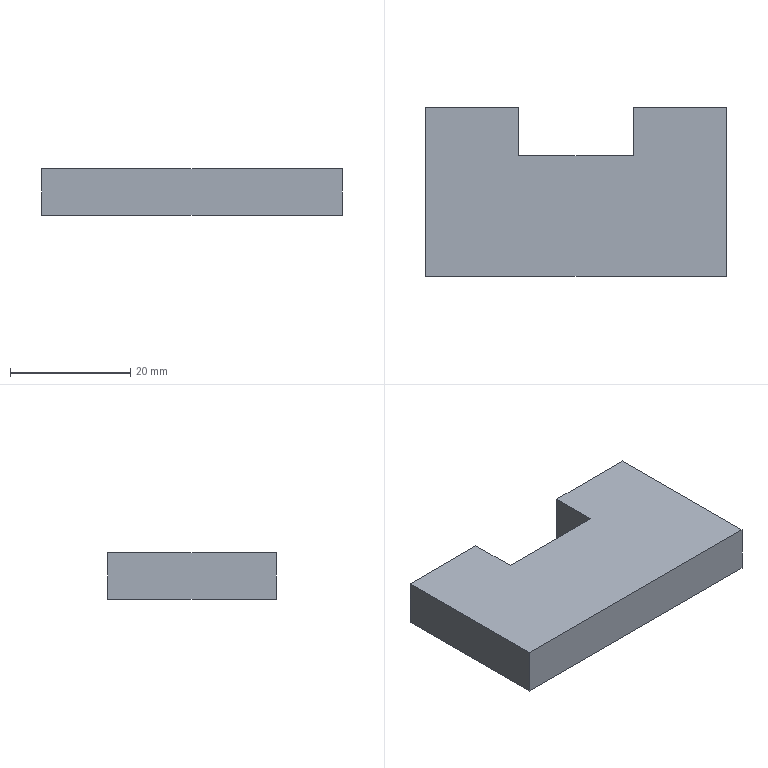Part | 1 solid | 10 faces | box 50 x 28 x 7.8 mm | volume 9734 mm3 | plane 10
STEP:
#1=CARTESIAN_POINT('',(25.,-14.,0.));
#2=VERTEX_POINT('',#1);
#3=CARTESIAN_POINT('',(25.,14.,0.));
#4=VERTEX_POINT('',#3);
#5=CARTESIAN_POINT('',(25.,14.,0.));
#6=DIRECTION('',(0.,1.,0.));
#7=VECTOR('',#6,1000.);
#8=LINE('',#5,#7);
#9=EDGE_CURVE('',#2,#4,#8,.T.);
#10=ORIENTED_EDGE('',*,*,#9,.F.);
#11=CARTESIAN_POINT('',(25.,-14.,-7.8));
#12=VERTEX_POINT('',#11);
#13=CARTESIAN_POINT('',(25.,-14.,-7.8));
#14=DIRECTION('',(0.,0.,1.));
#15=VECTOR('',#14,1000.);
#16=LINE('',#13,#15);
#17=EDGE_CURVE('',#12,#2,#16,.T.);
#18=ORIENTED_EDGE('',*,*,#17,.F.);
#19=CARTESIAN_POINT('',(25.,14.,-7.8));
#20=VERTEX_POINT('',#19);
#21=CARTESIAN_POINT('',(25.,14.,-7.8));
#22=DIRECTION('',(0.,1.,0.));
#23=VECTOR('',#22,1000.);
#24=LINE('',#21,#23);
#25=EDGE_CURVE('',#12,#20,#24,.T.);
#26=ORIENTED_EDGE('',*,*,#25,.T.);
#27=CARTESIAN_POINT('',(25.,14.,-7.8));
#28=DIRECTION('',(0.,0.,1.));
#29=VECTOR('',#28,1000.);
#30=LINE('',#27,#29);
#31=EDGE_CURVE('',#20,#4,#30,.T.);
#32=ORIENTED_EDGE('',*,*,#31,.T.);
#33=EDGE_LOOP('',(#10,#18,#26,#32));
#34=FACE_OUTER_BOUND('',#33,.T.);
#35=CARTESIAN_POINT('',(25.,14.,-7.8));
#36=DIRECTION('',(1.,0.,0.));
#37=DIRECTION('',(0.,1.,0.));
#38=AXIS2_PLACEMENT_3D('',#35,#36,#37);
#39=PLANE('',#38);
#40=ADVANCED_FACE('',(#34),#39,.T.);
#41=CARTESIAN_POINT('',(-25.,-14.,0.));
#42=VERTEX_POINT('',#41);
#43=CARTESIAN_POINT('',(-25.,-14.,0.));
#44=DIRECTION('',(1.,0.,0.));
#45=VECTOR('',#44,1000.);
#46=LINE('',#43,#45);
#47=EDGE_CURVE('',#42,#2,#46,.T.);
#48=ORIENTED_EDGE('',*,*,#47,.F.);
#49=CARTESIAN_POINT('',(-25.,-14.,-7.8));
#50=VERTEX_POINT('',#49);
#51=CARTESIAN_POINT('',(-25.,-14.,-7.8));
#52=DIRECTION('',(0.,0.,1.));
#53=VECTOR('',#52,1000.);
#54=LINE('',#51,#53);
#55=EDGE_CURVE('',#50,#42,#54,.T.);
#56=ORIENTED_EDGE('',*,*,#55,.F.);
#57=CARTESIAN_POINT('',(-25.,-14.,-7.8));
#58=DIRECTION('',(1.,0.,0.));
#59=VECTOR('',#58,1000.);
#60=LINE('',#57,#59);
#61=EDGE_CURVE('',#50,#12,#60,.T.);
#62=ORIENTED_EDGE('',*,*,#61,.T.);
#63=ORIENTED_EDGE('',*,*,#17,.T.);
#64=EDGE_LOOP('',(#48,#56,#62,#63));
#65=FACE_OUTER_BOUND('',#64,.T.);
#66=CARTESIAN_POINT('',(-25.,-14.,-7.8));
#67=DIRECTION('',(0.,-1.,0.));
#68=DIRECTION('',(0.,0.,-1.));
#69=AXIS2_PLACEMENT_3D('',#66,#67,#68);
#70=PLANE('',#69);
#71=ADVANCED_FACE('',(#65),#70,.T.);
#72=CARTESIAN_POINT('',(-25.,14.,0.));
#73=VERTEX_POINT('',#72);
#74=CARTESIAN_POINT('',(-25.,14.,0.));
#75=DIRECTION('',(0.,-1.,0.));
#76=VECTOR('',#75,1000.);
#77=LINE('',#74,#76);
#78=EDGE_CURVE('',#73,#42,#77,.T.);
#79=ORIENTED_EDGE('',*,*,#78,.F.);
#80=CARTESIAN_POINT('',(-25.,14.,-7.8));
#81=VERTEX_POINT('',#80);
#82=CARTESIAN_POINT('',(-25.,14.,-7.8));
#83=DIRECTION('',(0.,0.,1.));
#84=VECTOR('',#83,1000.);
#85=LINE('',#82,#84);
#86=EDGE_CURVE('',#81,#73,#85,.T.);
#87=ORIENTED_EDGE('',*,*,#86,.F.);
#88=CARTESIAN_POINT('',(-25.,14.,-7.8));
#89=DIRECTION('',(0.,-1.,0.));
#90=VECTOR('',#89,1000.);
#91=LINE('',#88,#90);
#92=EDGE_CURVE('',#81,#50,#91,.T.);
#93=ORIENTED_EDGE('',*,*,#92,.T.);
#94=ORIENTED_EDGE('',*,*,#55,.T.);
#95=EDGE_LOOP('',(#79,#87,#93,#94));
#96=FACE_OUTER_BOUND('',#95,.T.);
#97=CARTESIAN_POINT('',(-25.,14.,-7.8));
#98=DIRECTION('',(-1.,0.,0.));
#99=DIRECTION('',(0.,-1.,0.));
#100=AXIS2_PLACEMENT_3D('',#97,#98,#99);
#101=PLANE('',#100);
#102=ADVANCED_FACE('',(#96),#101,.T.);
#103=CARTESIAN_POINT('',(-9.5,14.,0.));
#104=VERTEX_POINT('',#103);
#105=CARTESIAN_POINT('',(-25.,14.,0.));
#106=DIRECTION('',(-1.,0.,0.));
#107=VECTOR('',#106,1000.);
#108=LINE('',#105,#107);
#109=EDGE_CURVE('',#104,#73,#108,.T.);
#110=ORIENTED_EDGE('',*,*,#109,.F.);
#111=CARTESIAN_POINT('',(-9.5,14.,-7.8));
#112=VERTEX_POINT('',#111);
#113=CARTESIAN_POINT('',(-9.5,14.,-7.8));
#114=DIRECTION('',(0.,0.,1.));
#115=VECTOR('',#114,1000.);
#116=LINE('',#113,#115);
#117=EDGE_CURVE('',#112,#104,#116,.T.);
#118=ORIENTED_EDGE('',*,*,#117,.F.);
#119=CARTESIAN_POINT('',(-25.,14.,-7.8));
#120=DIRECTION('',(-1.,0.,0.));
#121=VECTOR('',#120,1000.);
#122=LINE('',#119,#121);
#123=EDGE_CURVE('',#112,#81,#122,.T.);
#124=ORIENTED_EDGE('',*,*,#123,.T.);
#125=ORIENTED_EDGE('',*,*,#86,.T.);
#126=EDGE_LOOP('',(#110,#118,#124,#125));
#127=FACE_OUTER_BOUND('',#126,.T.);
#128=CARTESIAN_POINT('',(-25.,14.,-7.8));
#129=DIRECTION('',(0.,1.,0.));
#130=DIRECTION('',(0.,0.,1.));
#131=AXIS2_PLACEMENT_3D('',#128,#129,#130);
#132=PLANE('',#131);
#133=ADVANCED_FACE('',(#127),#132,.T.);
#134=CARTESIAN_POINT('',(-9.5,6.,0.));
#135=VERTEX_POINT('',#134);
#136=CARTESIAN_POINT('',(-9.5,14.,0.));
#137=DIRECTION('',(0.,1.,0.));
#138=VECTOR('',#137,1000.);
#139=LINE('',#136,#138);
#140=EDGE_CURVE('',#135,#104,#139,.T.);
#141=ORIENTED_EDGE('',*,*,#140,.F.);
#142=CARTESIAN_POINT('',(-9.5,6.,-7.8));
#143=VERTEX_POINT('',#142);
#144=CARTESIAN_POINT('',(-9.5,6.,-7.8));
#145=DIRECTION('',(0.,0.,1.));
#146=VECTOR('',#145,1000.);
#147=LINE('',#144,#146);
#148=EDGE_CURVE('',#143,#135,#147,.T.);
#149=ORIENTED_EDGE('',*,*,#148,.F.);
#150=CARTESIAN_POINT('',(-9.5,14.,-7.8));
#151=DIRECTION('',(0.,1.,0.));
#152=VECTOR('',#151,1000.);
#153=LINE('',#150,#152);
#154=EDGE_CURVE('',#143,#112,#153,.T.);
#155=ORIENTED_EDGE('',*,*,#154,.T.);
#156=ORIENTED_EDGE('',*,*,#117,.T.);
#157=EDGE_LOOP('',(#141,#149,#155,#156));
#158=FACE_OUTER_BOUND('',#157,.T.);
#159=CARTESIAN_POINT('',(-9.5,14.,-7.8));
#160=DIRECTION('',(1.,0.,0.));
#161=DIRECTION('',(0.,1.,0.));
#162=AXIS2_PLACEMENT_3D('',#159,#160,#161);
#163=PLANE('',#162);
#164=ADVANCED_FACE('',(#158),#163,.T.);
#165=CARTESIAN_POINT('',(9.5,6.,0.));
#166=VERTEX_POINT('',#165);
#167=CARTESIAN_POINT('',(-9.5,6.,0.));
#168=DIRECTION('',(-1.,0.,0.));
#169=VECTOR('',#168,1000.);
#170=LINE('',#167,#169);
#171=EDGE_CURVE('',#166,#135,#170,.T.);
#172=ORIENTED_EDGE('',*,*,#171,.F.);
#173=CARTESIAN_POINT('',(9.5,6.,-7.8));
#174=VERTEX_POINT('',#173);
#175=CARTESIAN_POINT('',(9.5,6.,-7.8));
#176=DIRECTION('',(0.,0.,1.));
#177=VECTOR('',#176,1000.);
#178=LINE('',#175,#177);
#179=EDGE_CURVE('',#174,#166,#178,.T.);
#180=ORIENTED_EDGE('',*,*,#179,.F.);
#181=CARTESIAN_POINT('',(-9.5,6.,-7.8));
#182=DIRECTION('',(-1.,0.,0.));
#183=VECTOR('',#182,1000.);
#184=LINE('',#181,#183);
#185=EDGE_CURVE('',#174,#143,#184,.T.);
#186=ORIENTED_EDGE('',*,*,#185,.T.);
#187=ORIENTED_EDGE('',*,*,#148,.T.);
#188=EDGE_LOOP('',(#172,#180,#186,#187));
#189=FACE_OUTER_BOUND('',#188,.T.);
#190=CARTESIAN_POINT('',(-9.5,6.,-7.8));
#191=DIRECTION('',(0.,1.,0.));
#192=DIRECTION('',(0.,0.,1.));
#193=AXIS2_PLACEMENT_3D('',#190,#191,#192);
#194=PLANE('',#193);
#195=ADVANCED_FACE('',(#189),#194,.T.);
#196=CARTESIAN_POINT('',(9.5,14.,0.));
#197=VERTEX_POINT('',#196);
#198=CARTESIAN_POINT('',(9.5,14.,0.));
#199=DIRECTION('',(0.,-1.,0.));
#200=VECTOR('',#199,1000.);
#201=LINE('',#198,#200);
#202=EDGE_CURVE('',#197,#166,#201,.T.);
#203=ORIENTED_EDGE('',*,*,#202,.F.);
#204=CARTESIAN_POINT('',(9.5,14.,-7.8));
#205=VERTEX_POINT('',#204);
#206=CARTESIAN_POINT('',(9.5,14.,-7.8));
#207=DIRECTION('',(0.,0.,1.));
#208=VECTOR('',#207,1000.);
#209=LINE('',#206,#208);
#210=EDGE_CURVE('',#205,#197,#209,.T.);
#211=ORIENTED_EDGE('',*,*,#210,.F.);
#212=CARTESIAN_POINT('',(9.5,14.,-7.8));
#213=DIRECTION('',(0.,-1.,0.));
#214=VECTOR('',#213,1000.);
#215=LINE('',#212,#214);
#216=EDGE_CURVE('',#205,#174,#215,.T.);
#217=ORIENTED_EDGE('',*,*,#216,.T.);
#218=ORIENTED_EDGE('',*,*,#179,.T.);
#219=EDGE_LOOP('',(#203,#211,#217,#218));
#220=FACE_OUTER_BOUND('',#219,.T.);
#221=CARTESIAN_POINT('',(9.5,14.,-7.8));
#222=DIRECTION('',(-1.,0.,0.));
#223=DIRECTION('',(0.,-1.,0.));
#224=AXIS2_PLACEMENT_3D('',#221,#222,#223);
#225=PLANE('',#224);
#226=ADVANCED_FACE('',(#220),#225,.T.);
#227=CARTESIAN_POINT('',(9.5,14.,0.));
#228=DIRECTION('',(-1.,0.,0.));
#229=VECTOR('',#228,1000.);
#230=LINE('',#227,#229);
#231=EDGE_CURVE('',#4,#197,#230,.T.);
#232=ORIENTED_EDGE('',*,*,#231,.F.);
#233=ORIENTED_EDGE('',*,*,#31,.F.);
#234=CARTESIAN_POINT('',(9.5,14.,-7.8));
#235=DIRECTION('',(-1.,0.,0.));
#236=VECTOR('',#235,1000.);
#237=LINE('',#234,#236);
#238=EDGE_CURVE('',#20,#205,#237,.T.);
#239=ORIENTED_EDGE('',*,*,#238,.T.);
#240=ORIENTED_EDGE('',*,*,#210,.T.);
#241=EDGE_LOOP('',(#232,#233,#239,#240));
#242=FACE_OUTER_BOUND('',#241,.T.);
#243=CARTESIAN_POINT('',(9.5,14.,-7.8));
#244=DIRECTION('',(0.,1.,0.));
#245=DIRECTION('',(0.,0.,1.));
#246=AXIS2_PLACEMENT_3D('',#243,#244,#245);
#247=PLANE('',#246);
#248=ADVANCED_FACE('',(#242),#247,.T.);
#249=ORIENTED_EDGE('',*,*,#25,.F.);
#250=ORIENTED_EDGE('',*,*,#61,.F.);
#251=ORIENTED_EDGE('',*,*,#92,.F.);
#252=ORIENTED_EDGE('',*,*,#123,.F.);
#253=ORIENTED_EDGE('',*,*,#154,.F.);
#254=ORIENTED_EDGE('',*,*,#185,.F.);
#255=ORIENTED_EDGE('',*,*,#216,.F.);
#256=ORIENTED_EDGE('',*,*,#238,.F.);
#257=EDGE_LOOP('',(#249,#250,#251,#252,#253,#254,#255,#256));
#258=FACE_OUTER_BOUND('',#257,.T.);
#259=CARTESIAN_POINT('',(0.,0.,-7.8));
#260=DIRECTION('',(0.,0.,1.));
#261=DIRECTION('',(1.,0.,0.));
#262=AXIS2_PLACEMENT_3D('',#259,#260,#261);
#263=PLANE('',#262);
#264=ADVANCED_FACE('',(#258),#263,.F.);
#265=ORIENTED_EDGE('',*,*,#9,.T.);
#266=ORIENTED_EDGE('',*,*,#231,.T.);
#267=ORIENTED_EDGE('',*,*,#202,.T.);
#268=ORIENTED_EDGE('',*,*,#171,.T.);
#269=ORIENTED_EDGE('',*,*,#140,.T.);
#270=ORIENTED_EDGE('',*,*,#109,.T.);
#271=ORIENTED_EDGE('',*,*,#78,.T.);
#272=ORIENTED_EDGE('',*,*,#47,.T.);
#273=EDGE_LOOP('',(#265,#266,#267,#268,#269,#270,#271,#272));
#274=FACE_OUTER_BOUND('',#273,.T.);
#275=CARTESIAN_POINT('',(0.,0.,0.));
#276=DIRECTION('',(0.,0.,1.));
#277=DIRECTION('',(1.,0.,0.));
#278=AXIS2_PLACEMENT_3D('',#275,#276,#277);
#279=PLANE('',#278);
#280=ADVANCED_FACE('',(#274),#279,.T.);
#281=CLOSED_SHELL('',(#40,#71,#102,#133,#164,#195,#226,#248,#264,#280));
#282=MANIFOLD_SOLID_BREP('',#281);
#283=CARTESIAN_POINT('',(0.,0.,0.));
#284=DIRECTION('',(0.,0.,1.));
#285=DIRECTION('',(1.,0.,0.));
#286=AXIS2_PLACEMENT_3D('',#283,#284,#285);
#287=(LENGTH_UNIT()NAMED_UNIT(*)SI_UNIT(.MILLI.,.METRE.));
#288=UNCERTAINTY_MEASURE_WITH_UNIT(LENGTH_MEASURE(0.00001),#287,'','');
#289=(NAMED_UNIT(*)PLANE_ANGLE_UNIT()SI_UNIT($,.RADIAN.));
#290=(NAMED_UNIT(*)SI_UNIT($,.STERADIAN.)SOLID_ANGLE_UNIT());
#291=(GEOMETRIC_REPRESENTATION_CONTEXT(3)GLOBAL_UNCERTAINTY_ASSIGNED_CONTEXT((#288))GLOBAL_UNIT_ASSIGNED_CONTEXT((#287,#289,#290))REPRESENTATION_CONTEXT('',''));
#292=ADVANCED_BREP_SHAPE_REPRESENTATION('',(#282,#286),#291);